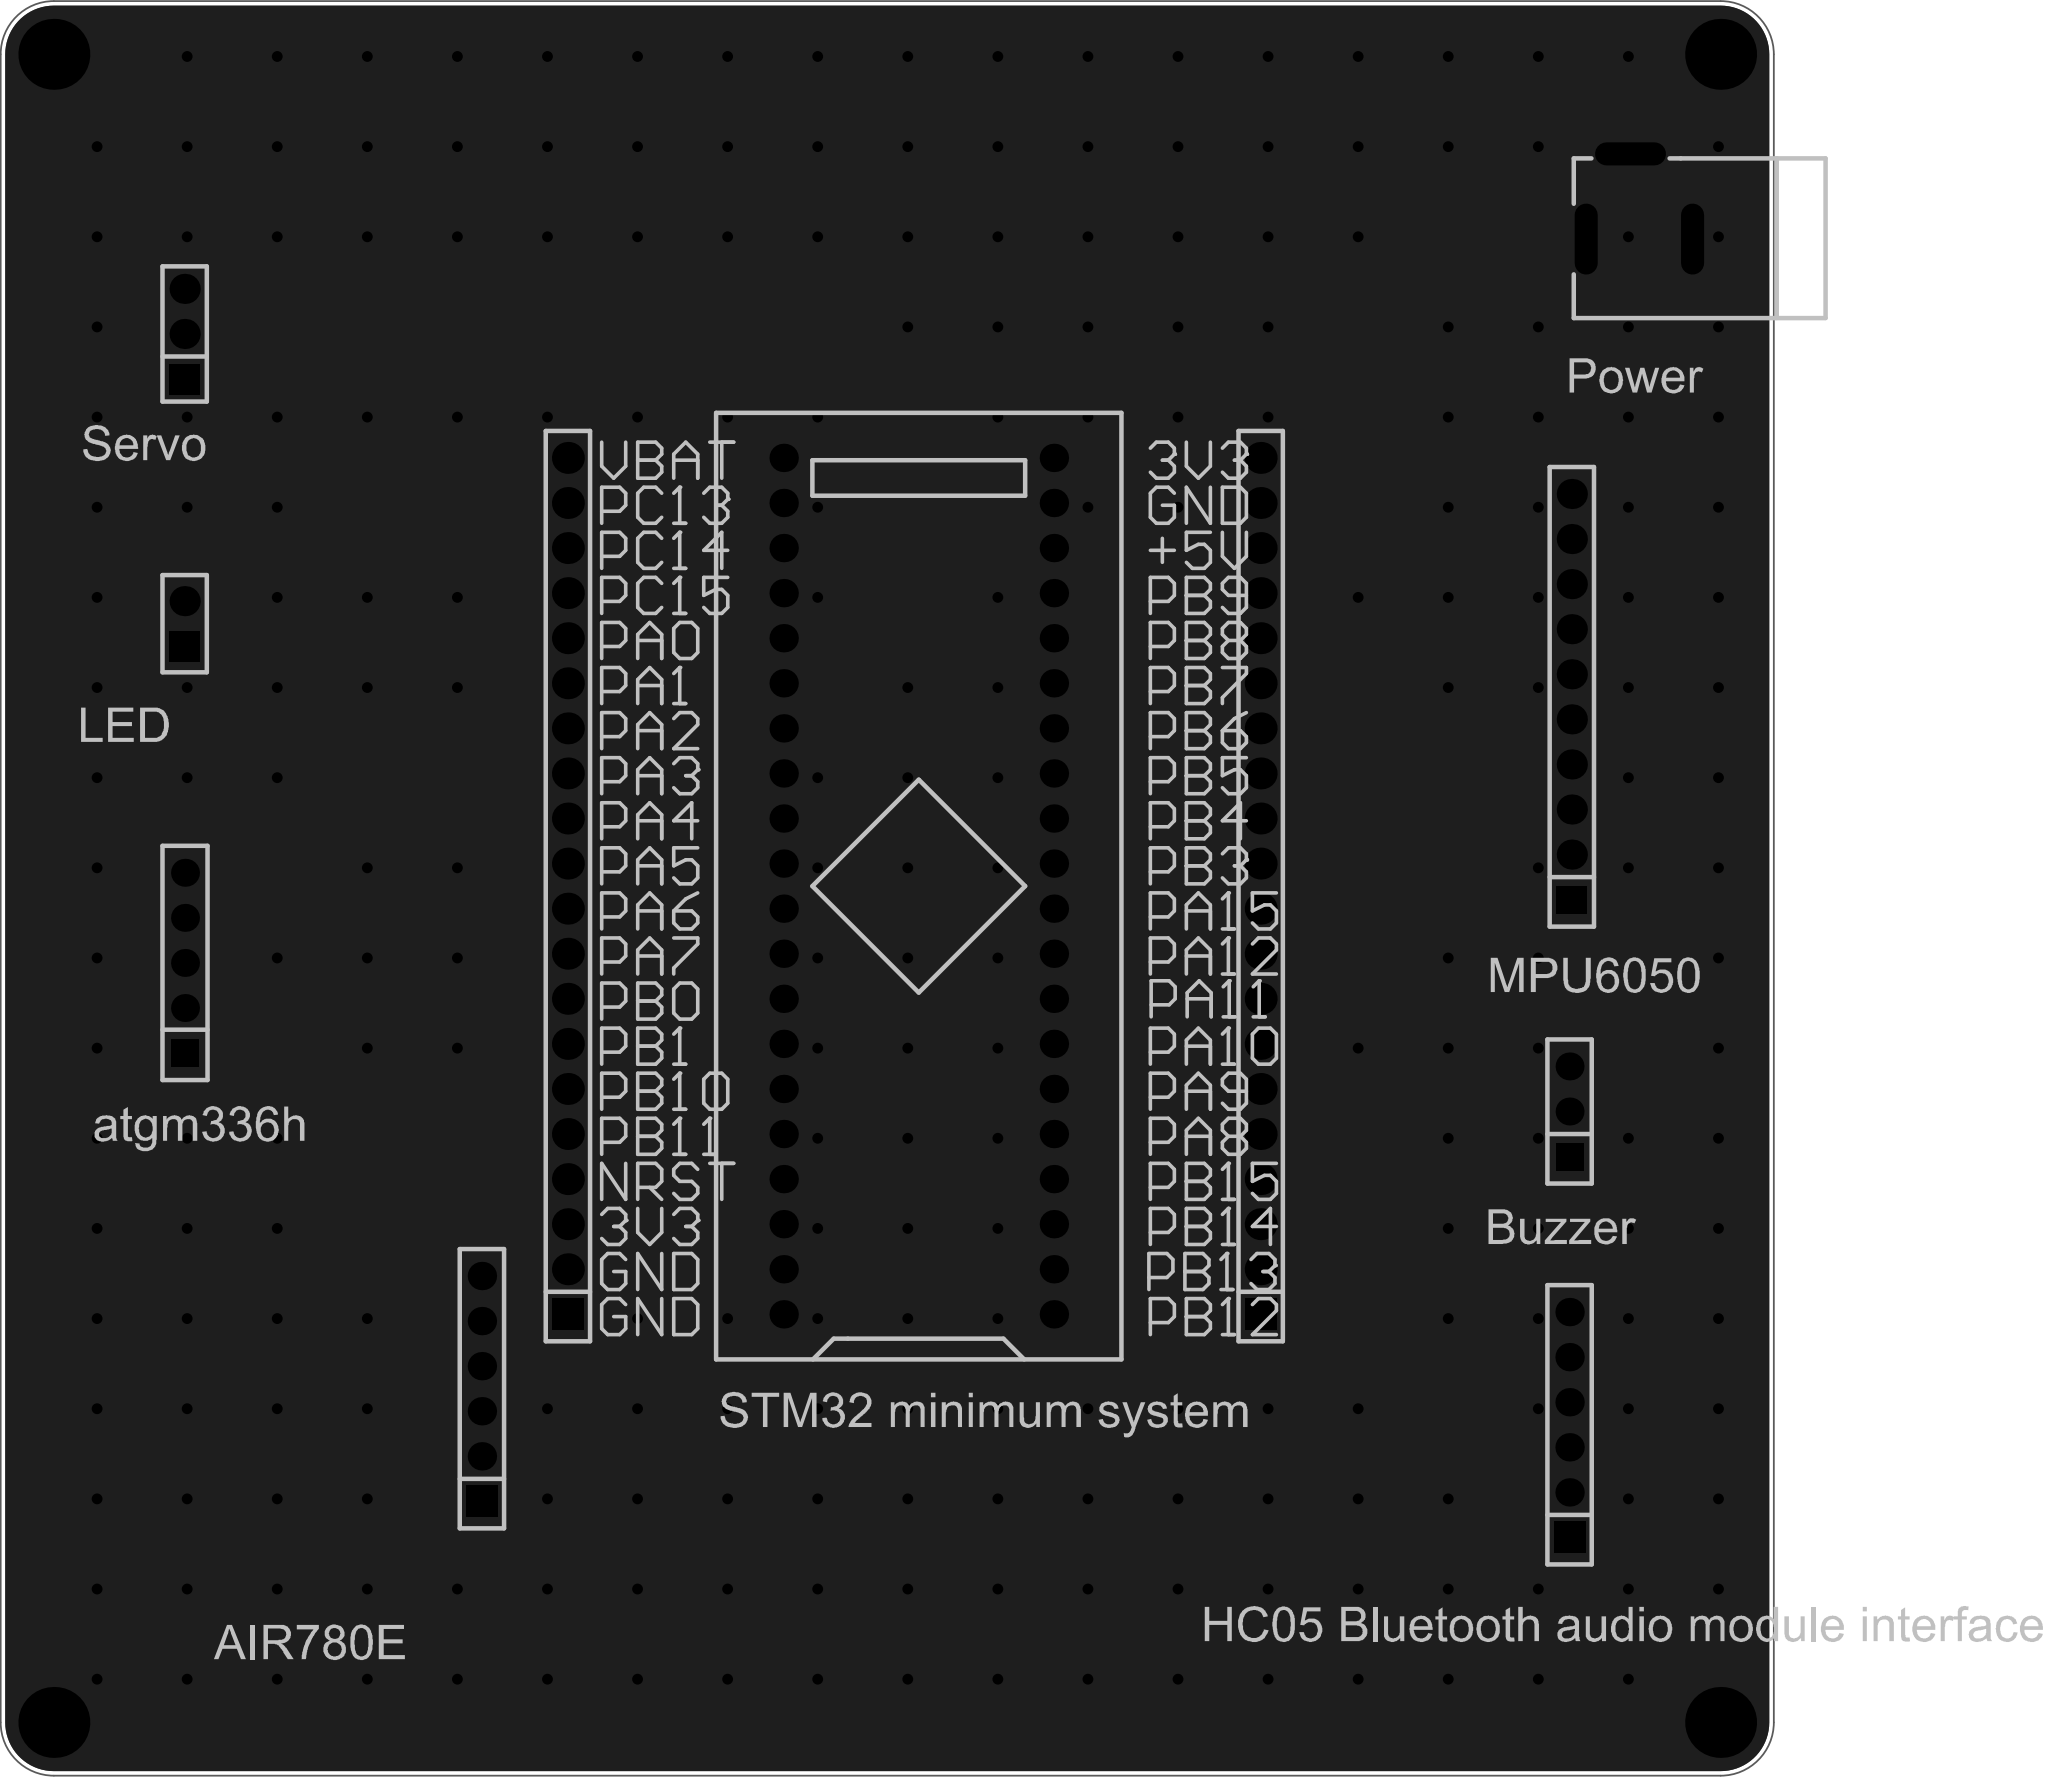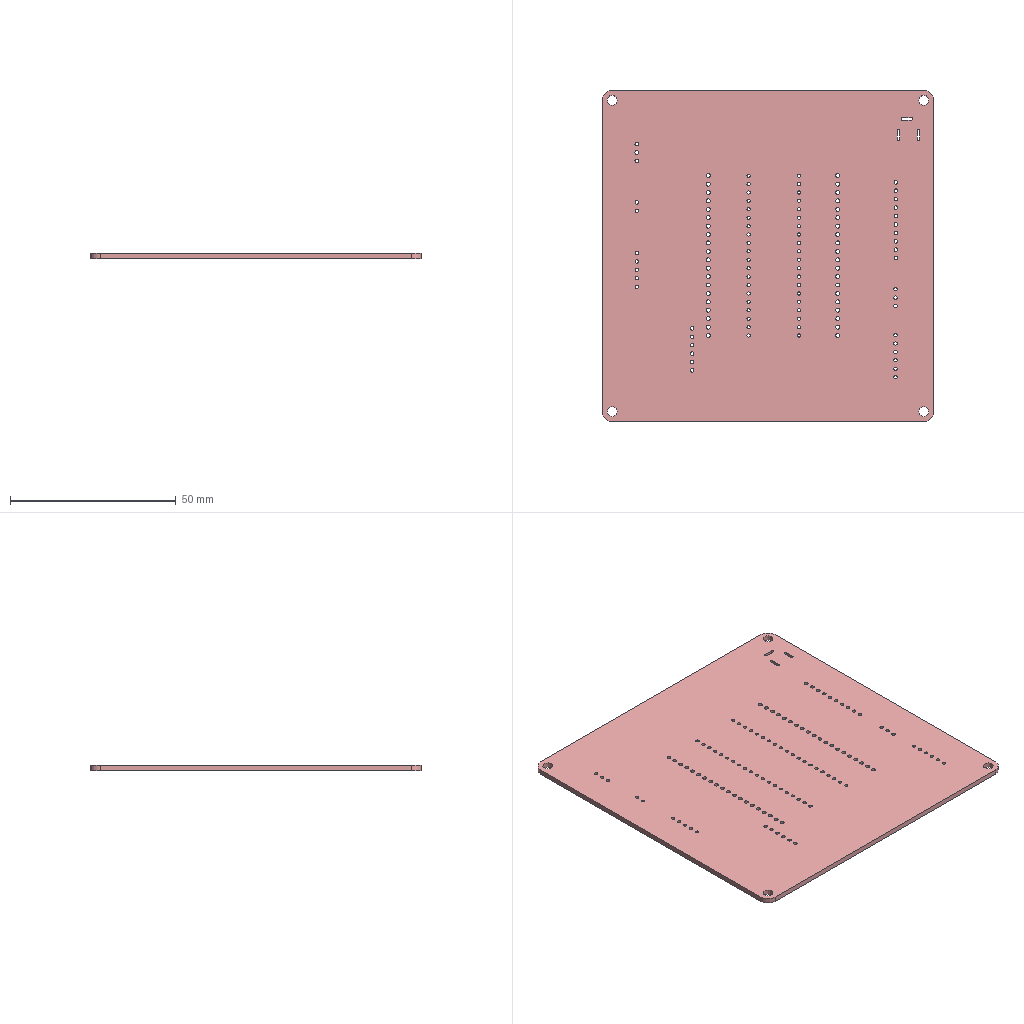Circuit board layout | Altium Designer | box 100 x 100 x 1.6 mm
Layer stack:
# Altium Designer layer stack of  (unit mm; dielectric type: 0 none, 1 core, 2 prepreg, 3 surface material)
index,name,kind,layer,copper_thickness_mm,dielectric_type,dielectric_thickness_mm,dielectric_material,dielectric_constant
0,Top Paste Mask Layer,other,,,,,,
1,Top Silkscreen Layer,other,,,,,,
2,Top Solder Mask Layer,dielectric,,,3,0.01,,3.3
3,Top Layer,copper,Top Layer,0.035,,,,
4,Dielectric1,dielectric,,,3,1.51,FR4,4.5
5,Bottom Layer,copper,Bottom Layer,0.035,,,,
6,Bottom Solder Mask Layer,dielectric,,,3,0.01,,3.3
7,Bottom Silkscreen Layer,other,,,,,,
8,Bottom Paste Mask Layer,other,,,,,,
# drill layer pairs: low layer,high layer
drill_pair,Top Layer,Bottom Layer
Part placement:
Designator,Comment,Layer,Footprint,Center-X(mm),Center-Y(mm),Rotation
U1,STM32F103C8T6-Card,TopLayer,CONN-TH_L53.3-W22.9_STM32F103C8T6-CARD,132.334,129.032,90
H1,,TopLayer,HDR-TH_20P-P2.54-V-F,151.617,129.032,90
H2,,TopLayer,HDR-TH_20P-P2.54-V-F,112.546,129.032,90
DC1,,TopLayer,DC-2.0,172.974,167.894,0
H4,,TopLayer,HDR-TH_6P-P2.54-V-F,169.037,98.679,90
H5,,TopLayer,HDR-TH_3P-P2.54-V-F,169.037,116.332,90
H3,,TopLayer,HDR-TH_6P-P2.54-V-F,107.696,100.711,90
H6,,TopLayer,HDR-TH_5P-P2.54-V-F,90.952,124.704,90
H7,,TopLayer,HDR-TH_10P-P2.54-V-F,169.164,139.7,90
H8,,TopLayer,HDR-TH_3P-P2.54-V-M,90.932,160.147,90
H9,,TopLayer,HDR-TH_2P-P2.54-V-F,90.932,143.82,90
Pad and via stacks:
# Altium Designer via and pad stacks of  (unit mm). Each distinct definition once, with the count of objects using it.
# via: kind,start_layer,end_layer,hole_mm,diameter_mm,mode(0 simple;1 top-mid-bottom;2 full stack),diameter_per_layer,count,example_net
# pad: kind,layer,hole_mm,hole_type(0 round;1 square;2 slot),plating,top_size,top_shape(1 round;2 rect;3 octagon;9 rounded rect),mid_size,bottom_size,mode,footprint,size_per_layer,count,example
pad,Multi-Layer,3,0,plated,4x4,1,4x4,4x4,0,,,4,1
pad,Multi-Layer,1,0,plated,1.6x1.6,1,1.6x1.6,1.6x1.6,0,CONN-TH_L53.3-W22.9_STM32F103C8T6-CARD,,40,U1.1
pad,Multi-Layer,1.2,0,plated,1.8x1.8,2,1.8x1.8,1.8x1.8,0,HDR-TH_20P-P2.54-V-F,,2,H1.1
pad,Multi-Layer,1.2,0,plated,1.8x1.8,1,1.8x1.8,1.8x1.8,0,HDR-TH_20P-P2.54-V-F,,38,H1.2
pad,Multi-Layer,0.8001,2,plated,4x1.3,1,4x1.3,4x1.3,0,DC-2.0,,3,DC1.2
pad,Multi-Layer,1.02,0,plated,1.6x1.6,1,1.6x1.6,1.6x1.6,0,HDR-TH_6P-P2.54-V-F,,10,H4.6
pad,Multi-Layer,1.02,0,plated,1.8x1.8,2,1.8x1.8,1.8x1.8,0,HDR-TH_6P-P2.54-V-F,,2,H4.1
pad,Multi-Layer,1.02,0,plated,1.575x1.575,1,1.575x1.575,1.575x1.575,0,HDR-TH_3P-P2.54-V-F,,2,H5.3
pad,Multi-Layer,1.02,0,plated,1.575x1.575,2,1.575x1.575,1.575x1.575,0,HDR-TH_3P-P2.54-V-F,,1,H5.1
pad,Multi-Layer,1.02,0,plated,1.575x1.575,1,1.575x1.575,1.575x1.575,0,HDR-TH_5P-P2.54-V-F,,4,H6.5
pad,Multi-Layer,1.02,0,plated,1.575x1.575,2,1.575x1.575,1.575x1.575,0,HDR-TH_5P-P2.54-V-F,,1,H6.1
pad,Multi-Layer,1.1,0,plated,1.7x1.7,1,1.7x1.7,1.7x1.7,0,HDR-TH_10P-P2.54-V-F,,9,H7.10
pad,Multi-Layer,1.1,0,plated,1.575x1.7,2,1.575x1.7,1.575x1.7,0,HDR-TH_10P-P2.54-V-F,,1,H7.1
pad,Multi-Layer,1.1,0,plated,1.7x1.7,2,1.7x1.7,1.7x1.7,0,HDR-TH_3P-P2.54-V-M,,1,H8.1
pad,Multi-Layer,1.1,0,plated,1.7x1.7,1,1.7x1.7,1.7x1.7,0,HDR-TH_3P-P2.54-V-M,,2,H8.2
pad,Multi-Layer,1,0,plated,1.7x1.7,2,1.7x1.7,1.7x1.7,0,HDR-TH_2P-P2.54-V-F,,1,H9.1
pad,Multi-Layer,1,0,plated,1.7x1.7,1,1.7x1.7,1.7x1.7,0,HDR-TH_2P-P2.54-V-F,,1,H9.2
via,Top Layer,Bottom Layer,0.3048,0.61,0,,252,GND
Copper pours:
name,layer,net,type(0 solid;1 hatched;2 none)
Bottom Layer-GND,Bottom Layer,GND,0
Top Layer-GND,Top Layer,GND,0